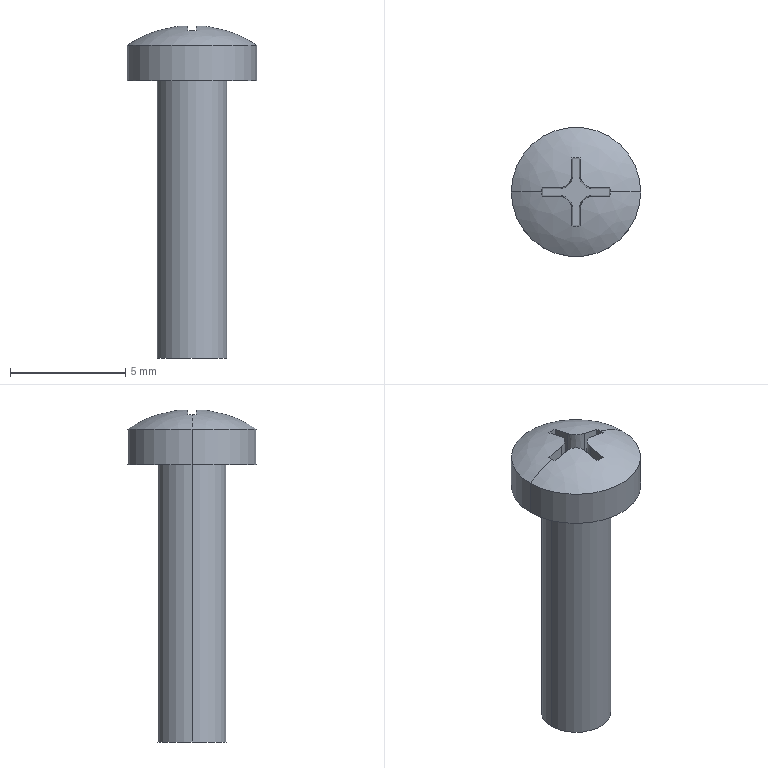Part | STEP file | GB818-M3X12-ZN-4.8_1 | 1 solid | 26 faces | box 5.6 x 5.6 x 14.376 mm | volume 130.712 mm3 | plane 11 | cone 9 | cylinder 4 | spline 2 | commonest cylinder face diameters 3 x2 5.6 x2